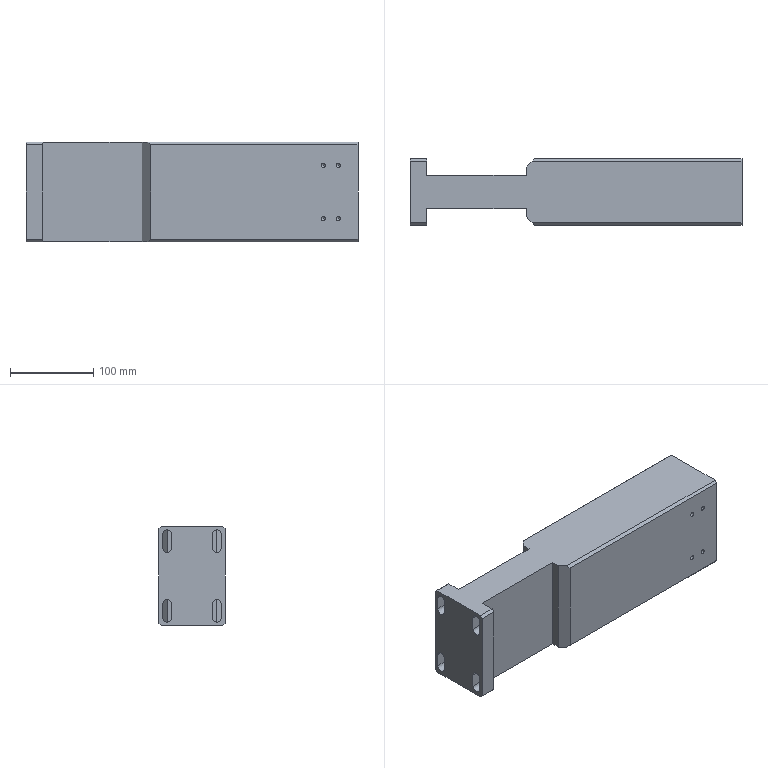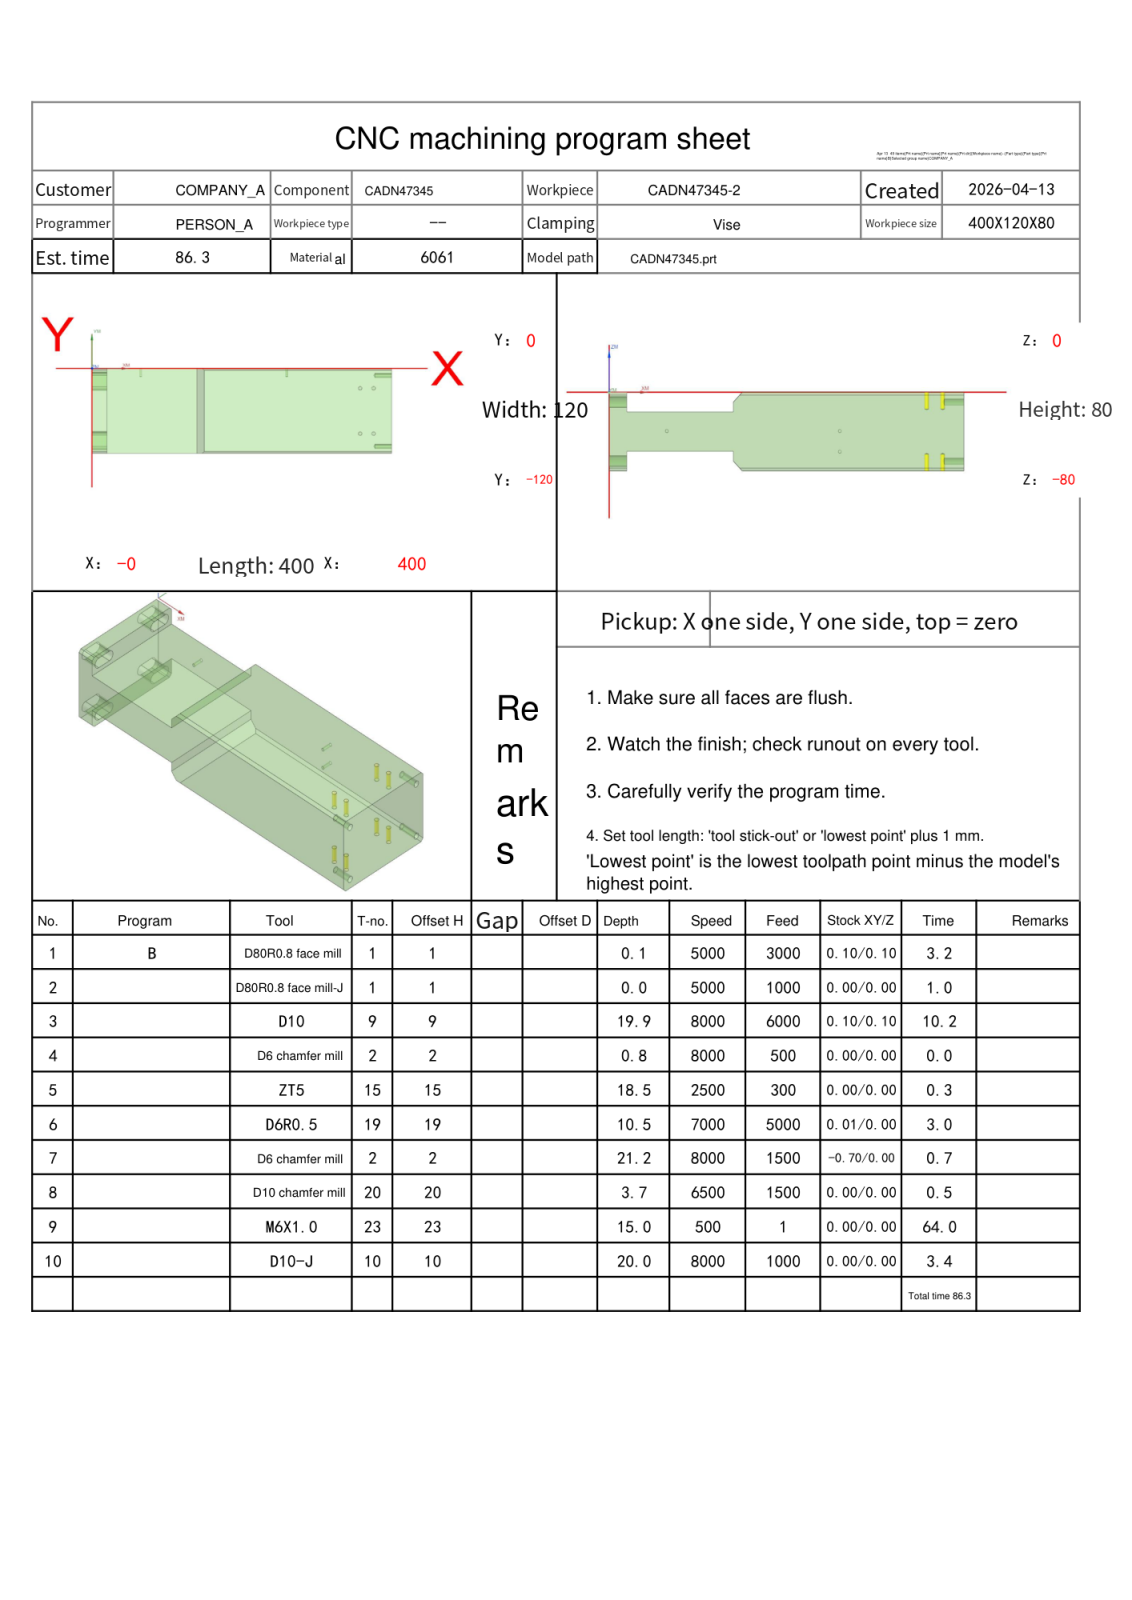NC program | NX | posted by the shop | part box 400 x 80 x 120 mm
Lines 1 to 147 of 4568:
%
O0001
(Machine time: 148.39 MIN)
(===Total Tool:8===)
(T1=D80R0.8 face mill D=80.  R=0.8  D-  H01 Z=-0.   )
(T9=D10     D=10.  R=0.   D-  H09 Z=-19.9 )
(T2=D6 chamfer mill   D=6.   R=0.   D-  H02 Z=-21.2 )
(T15=ZT5    D=5.   DR_a=118 D-  H15 Z=-18.5 )
(T19=D6R0.5 D=6.   R=0.5  D-  H19 Z=-10.5 )
(T20=D10 chamfer mill D=10.  R=0.  D-  H20 Z=-3.7  )
(T23=M6X1.0 D=5.   DR_a=180 D-  H23 Z=-15.  )
(T10=D10-J  D=10.  R=0.   D10 H10 Z=-20.  )
G80 G90 G17 G49 G40
G91 G28 Z0
M01
N1 T01 M06
(D80R0.8 face mill  D=80. R=0.8 H=01 ce=0.10 di=0.10)
G00 G90 G54 X452.097 Y-96.097 M03 S5000
G43 H01 Z20.
M08
Z6.011
G01 Z4.011 F3000.
X440.097
X-32.101
G02 X-40.097 Y-88.101 I.004 J8.
G01 Y-39.259
G02 X-32.101 Y-31.263 I8. J-.004
G01 X440.097
X452.097
Z6.011
G00 Y-96.097
Z5.522
G01 Z3.522
X440.097
X-32.101
G02 X-40.097 Y-88.101 I.004 J8.
G01 Y-39.259
G02 X-32.101 Y-31.263 I8. J-.004
G01 X440.097
X452.097
Z5.522
G00 Y-96.097
Z5.033
G01 Z3.033
X440.097
X-32.101
G02 X-40.097 Y-88.101 I.004 J8.
G01 Y-39.259
G02 X-32.101 Y-31.263 I8. J-.004
G01 X440.097
X452.097
Z5.033
G00 Y-96.097
Z4.544
G01 Z2.544
X440.097
X-32.101
G02 X-40.097 Y-88.101 I.004 J8.
G01 Y-39.259
G02 X-32.101 Y-31.263 I8. J-.004
G01 X440.097
X452.097
Z4.544
G00 Y-96.097
Z4.056
G01 Z2.056
X440.097
X-32.101
G02 X-40.097 Y-88.101 I.004 J8.
G01 Y-39.259
G02 X-32.101 Y-31.263 I8. J-.004
G01 X440.097
X452.097
Z4.056
G00 Y-96.097
Z3.567
G01 Z1.567
X440.097
X-32.101
G02 X-40.097 Y-88.101 I.004 J8.
G01 Y-39.259
G02 X-32.101 Y-31.263 I8. J-.004
G01 X440.097
X452.097
Z3.567
G00 Y-96.097
Z3.078
G01 Z1.078
X440.097
X-32.101
G02 X-40.097 Y-88.101 I.004 J8.
G01 Y-39.259
G02 X-32.101 Y-31.263 I8. J-.004
G01 X440.097
X452.097
Z3.078
G00 Y-96.097
Z2.589
G01 Z.589
X440.097
X-32.101
G02 X-40.097 Y-88.101 I.004 J8.
G01 Y-39.259
G02 X-32.101 Y-31.263 I8. J-.004
G01 X440.097
X452.097
Z2.589
G00 Y-96.097
Z2.1
G01 Z.1
X440.097
X-32.101
G02 X-40.097 Y-88.101 I.004 J8.
G01 Y-39.259
G02 X-32.101 Y-31.263 I8. J-.004
G01 X440.097
X452.097
Z2.1
G00 Z20.
G91 G28 Z0.0
M05
M09
G91 G28 Z0.0
M01
N2 T01 M06
(D80R0.8 face mill-J  D=80. R=0.8 H=01 ce=0.00 di=0.00)
G00 G90 G54 X451.999 Y-95.999 M03 S5000
G43 H01 Z20.
M08
Z2.
G01 Z0.0 F1000.
X439.999
X-32.003
G02 X-39.999 Y-88.003 I.004 J8.
G01 Y-39.356
G02 X-32.003 Y-31.361 I8. J-.005
G01 X439.999
X451.999
Z2.
G00 Z20.
G91 G28 Z0.0
M05
M09
G91 G28 Z0.0
M01